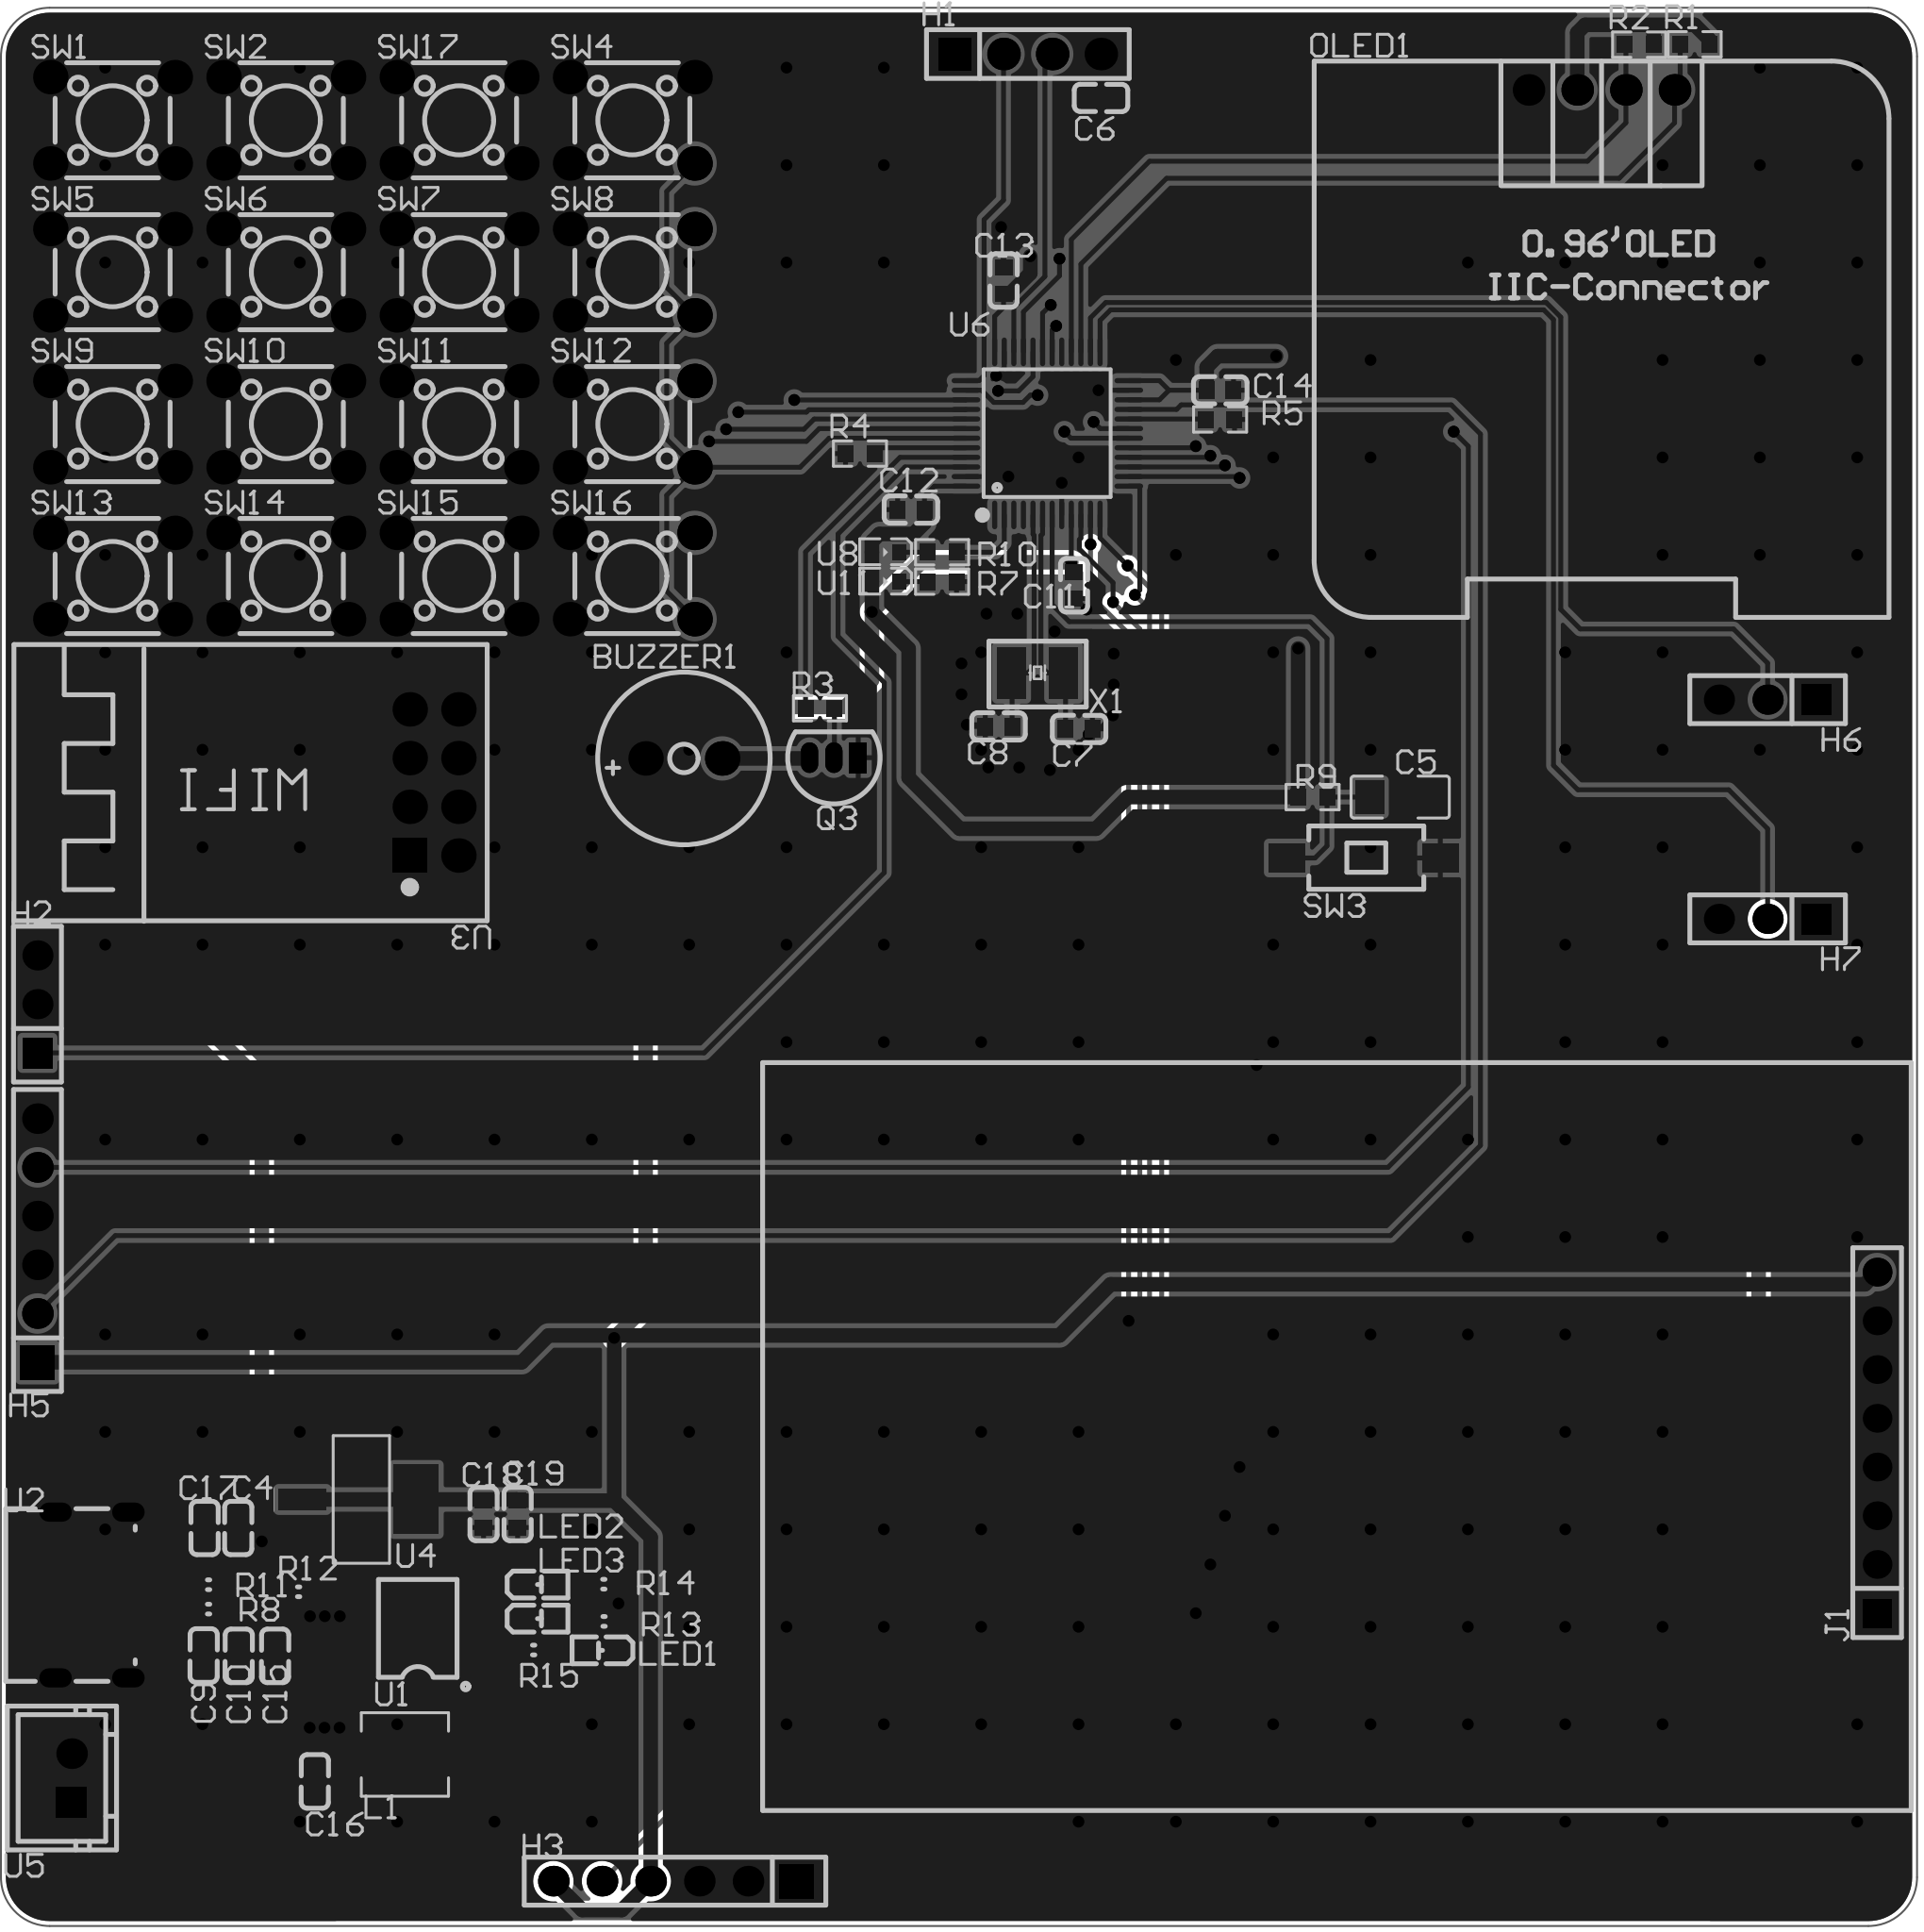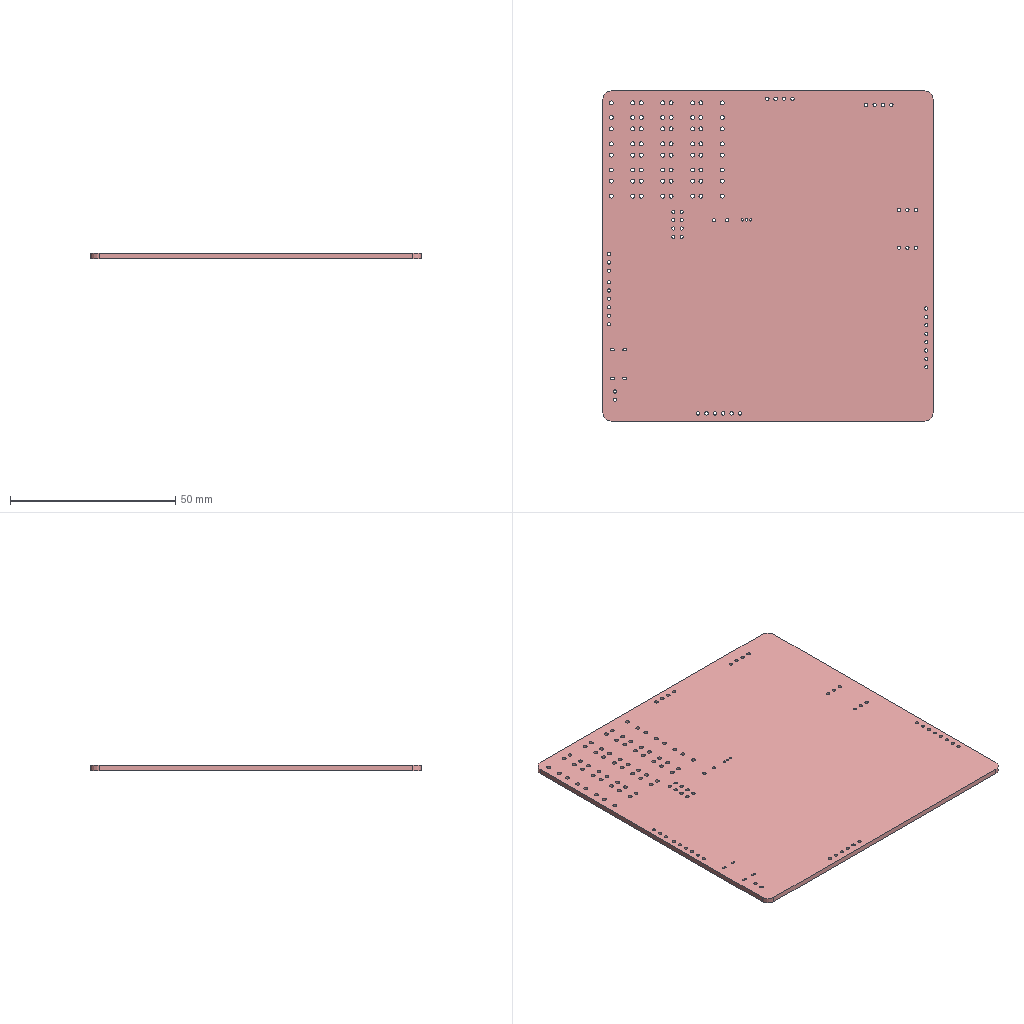Circuit board layout | Altium Designer | box 100 x 100 x 1.6 mm
Layer stack:
# Altium Designer layer stack of  (unit mm; dielectric type: 0 none, 1 core, 2 prepreg, 3 surface material)
index,name,kind,layer,copper_thickness_mm,dielectric_type,dielectric_thickness_mm,dielectric_material,dielectric_constant
0,Top Paste Mask Layer,other,,,,,,
1,Top Silkscreen Layer,other,,,,,,
2,Top Solder Mask Layer,dielectric,,,3,0.01,,3.3
3,Top Layer,copper,Top Layer,0.035,,,,
4,Dielectric1,dielectric,,,3,1.51,FR4,4.5
5,Bottom Layer,copper,Bottom Layer,0.035,,,,
6,Bottom Solder Mask Layer,dielectric,,,3,0.01,,3.3
7,Bottom Silkscreen Layer,other,,,,,,
8,Bottom Paste Mask Layer,other,,,,,,
# drill layer pairs: low layer,high layer
drill_pair,Top Layer,Bottom Layer
Part placement:
Designator,Comment,Layer,Footprint,Center-X(mm),Center-Y(mm),Rotation
BUZZER1,2.7kHz,TopLayer,BUZ-TH_BD9.0-P4.00-D0.6-FD,115.399,144.382,0
C4,10uF,TopLayer,C0603,92.139,104.263,270
C5,100uF,TopLayer,C1206,152.781,142.367,180
C6,100nF,TopLayer,C0603,137.16,178.816,180
C7,20pF,TopLayer,C0603,136.017,145.923,180
C8,20pF,TopLayer,C0603,131.826,146.05,0
C9,22uF,TopLayer,C0603,90.337,97.623,90
C10,22uF,TopLayer,C0603,92.167,97.605,90
C11,100nF,TopLayer,C0603,135.763,153.416,90
C12,100nF,TopLayer,C0603,127.254,157.353,0
C13,100nF,TopLayer,C0603,132.08,169.291,270
C14,100nF,TopLayer,C0603,143.383,163.576,180
C15,22uF,TopLayer,C0603,94.066,97.605,90
C16,22uF,TopLayer,C0603,96.139,91.059,90
C17,100nF,TopLayer,C0603,90.383,104.263,270
C18,10uF,TopLayer,C0603,104.942,104.989,90
C19,100nF,TopLayer,C0603,106.72,104.989,90
H1,,TopLayer,HDR-TH_4P-P2.54-V-F,133.35,181.102,0
H2,,TopLayer,HDR-TH_3P-P2.54-V-F,81.661,131.572,90
H3,,TopLayer,HDR-TH_6P-P2.54-V-F,114.935,85.852,180
H5,,TopLayer,HDR-TH_6P-P2.54-V-F,81.661,119.253,90
J1,,TopLayer,HDR-TH_8P-P2.54-V-M,177.673,108.712,90
L1,2.2uH,TopLayer,IND-SMD_L4.4-W4.2,100.838,92.456,180
LED1,Battery,TopLayer,LED0603_L1.6-W0.8-RD_BLUE,111.033,97.885,180
LED2,Discharge,TopLayer,LED0603_L1.6-W0.8-RD_BLUE,107.874,101.316,0
LED3,Charge,TopLayer,LED0603_L1.6-W0.8-RD_BLUE,107.874,99.538,0
OLED1,,TopLayer,0.96OLED_4P,163.291,179.234,0
Q3,,TopLayer,S8050_TO_92,123.226,144.422,180
R1,5.1K,TopLayer,R0603,168.148,181.61,0
R2,5.1K,TopLayer,R0603,165.252,181.593,0
R4,10kΩ,TopLayer,R0603,124.587,160.274,0
R5,10kΩ,TopLayer,R0603,143.383,162.052,180
R7,510Ω,TopLayer,R0603,128.875,153.599,0
R8,5.1K,TopLayer,R0603-NSK,90.591,100.036,180
R9,1kΩ,TopLayer,R0603,148.209,142.367,180
R10,510Ω,TopLayer,R0603,128.875,155.131,0
R11,5.1K,TopLayer,R0603-NSK,90.591,101.306,180
R12,56K,TopLayer,R0603-NSK,95.29,100.937,180
R13,5.1K,TopLayer,R0603-NSK,111.232,99.394,180
R14,5.1K,TopLayer,R0603-NSK,111.218,101.333,180
R15,5.1K,TopLayer,R0603-NSK,107.557,97.901,180
SW1,KH-6X6X6H-TJ,TopLayer,SW-TH_4P-L6.0-W6.0-P4.50-LS6.5,85.583,177.649,0
SW2,KH-6X6X6H-TJ,TopLayer,SW-TH_4P-L6.0-W6.0-P4.50-LS6.5,94.624,177.649,0
SW3,TS-1101-C-W,TopLayer,SW-SMD_L6.0-W3.3-LS8.0,150.876,139.192,180
SW4,KH-6X6X6H-TJ,TopLayer,SW-TH_4P-L6.0-W6.0-P4.50-LS6.5,112.707,177.649,0
SW5,KH-6X6X6H-TJ,TopLayer,SW-TH_4P-L6.0-W6.0-P4.50-LS6.5,85.583,169.73,0
SW6,KH-6X6X6H-TJ,TopLayer,SW-TH_4P-L6.0-W6.0-P4.50-LS6.5,94.624,169.73,0
SW7,KH-6X6X6H-TJ,TopLayer,SW-TH_4P-L6.0-W6.0-P4.50-LS6.5,103.666,169.73,0
SW8,KH-6X6X6H-TJ,TopLayer,SW-TH_4P-L6.0-W6.0-P4.50-LS6.5,112.707,169.73,0
SW9,KH-6X6X6H-TJ,TopLayer,SW-TH_4P-L6.0-W6.0-P4.50-LS6.5,85.583,161.81,0
SW10,KH-6X6X6H-TJ,TopLayer,SW-TH_4P-L6.0-W6.0-P4.50-LS6.5,94.624,161.81,0
SW11,KH-6X6X6H-TJ,TopLayer,SW-TH_4P-L6.0-W6.0-P4.50-LS6.5,103.666,161.81,0
SW12,KH-6X6X6H-TJ,TopLayer,SW-TH_4P-L6.0-W6.0-P4.50-LS6.5,112.707,161.81,0
SW13,KH-6X6X6H-TJ,TopLayer,SW-TH_4P-L6.0-W6.0-P4.50-LS6.5,85.583,153.892,0
SW14,KH-6X6X6H-TJ,TopLayer,SW-TH_4P-L6.0-W6.0-P4.50-LS6.5,94.624,153.892,0
SW15,KH-6X6X6H-TJ,TopLayer,SW-TH_4P-L6.0-W6.0-P4.50-LS6.5,103.666,153.892,0
SW16,KH-6X6X6H-TJ,TopLayer,SW-TH_4P-L6.0-W6.0-P4.50-LS6.5,112.707,153.892,0
SW17,KH-6X6X6H-TJ,TopLayer,SW-TH_4P-L6.0-W6.0-P4.50-LS6.5,103.666,177.649,0
U1,ETA9742,TopLayer,ESOP-8_L4.9-W3.9-P1.27-LS6.0-BL-EP,101.508,99.03,90
U2,YTC-TC6-268,TopLayer,TYPE-C-SMD_YIYUAN_YTC-TC6-268,84.731,100.77,270
U4,AMS1117-3.3,TopLayer,SOT-223-3_L6.5-W3.4-P2.30-LS7.0-BR,98.465,105.751,180
U6,STM32F103C8T6,TopLayer,LQFP-48_L7.0-W7.0-P0.50-LS9.0-BL,134.367,161.326,0
U8,42-51/GHC-YW2X2K/3T,TopLayer,LED-SMD_L1.6-W0.8-FD_GREEN-1,125.925,155.131,0
U11,42-51/GHC-YW2X2K/3T,TopLayer,LED-SMD_L1.6-W0.8-FD_GREEN-1,125.925,153.599,0
X1,8MHz,TopLayer,CRYSTAL-SMD_L3.2-W2.5_3225-8MHZ,133.858,148.844,180
R3,1K,TopLayer,R0603,122.501,146.998,180
U5,_x001F_XH2.54-2P,TopLayer,CONN-TH_2P-P2.54-V,83.445,91.23,90
H6,,TopLayer,HDR-TH_3P-P2.54-V-F,171.958,147.447,180
H7,,TopLayer,HDR-TH_3P-P2.54-V-F,171.958,136.017,180
U3,2.4GHz,TopLayer,WIFIM-TH_8P-L24.7-W14.4-P2.54,102.362,143.129,180
Pad and via stacks:
# Altium Designer via and pad stacks of  (unit mm). Each distinct definition once, with the count of objects using it.
# via: kind,start_layer,end_layer,hole_mm,diameter_mm,mode(0 simple;1 top-mid-bottom;2 full stack),diameter_per_layer,count,example_net
# pad: kind,layer,hole_mm,hole_type(0 round;1 square;2 slot),plating,top_size,top_shape(1 round;2 rect;3 octagon;9 rounded rect),mid_size,bottom_size,mode,footprint,size_per_layer,count,example
pad,Multi-Layer,1,0,plated,1.8x1.8,1,1.8x1.8,1.8x1.8,0,BUZ-TH_BD9.0-P4.00-D0.6-FD,,2,BUZZER1.1
pad,Multi-Layer,1.1,0,plated,1.7x1.7,2,1.7x1.7,1.7x1.7,0,HDR-TH_4P-P2.54-V-F,,1,H1.1
pad,Multi-Layer,1.1,0,plated,1.7x1.7,1,1.7x1.7,1.7x1.7,0,HDR-TH_4P-P2.54-V-F,,3,H1.2
pad,Multi-Layer,1.02,0,plated,1.575x1.575,1,1.575x1.575,1.575x1.575,0,HDR-TH_3P-P2.54-V-F,,6,H2.3
pad,Multi-Layer,1.02,0,plated,1.575x1.575,2,1.575x1.575,1.575x1.575,0,HDR-TH_3P-P2.54-V-F,,3,H2.1
pad,Multi-Layer,1.02,0,plated,1.6x1.6,1,1.6x1.6,1.6x1.6,0,HDR-TH_6P-P2.54-V-F,,10,H3.6
pad,Multi-Layer,1.02,0,plated,1.8x1.8,2,1.8x1.8,1.8x1.8,0,HDR-TH_6P-P2.54-V-F,,2,H3.1
pad,Multi-Layer,1,0,plated,1.5x1.5,2,1.5x1.5,1.5x1.5,0,HDR-TH_8P-P2.54-V-M,,1,J1.1
pad,Multi-Layer,1,0,plated,1.5x1.5,1,1.5x1.5,1.5x1.5,0,HDR-TH_8P-P2.54-V-M,,7,J1.2
pad,Multi-Layer,1,0,plated,1.65x1.65,1,1.65x1.65,1.65x1.65,0,0.96OLED_4P,,4,OLED1.4
pad,Multi-Layer,0.701,0,plated,0.8992x1.6,2,0.8992x1.6,0.8992x1.6,0,S8050_TO_92,,1,Q3.1
pad,Multi-Layer,0.701,0,plated,0.8992x1.6,1,0.8992x1.6,0.8992x1.6,0,S8050_TO_92,,2,Q3.2
pad,Multi-Layer,1.2,0,plated,1.8x1.8,1,1.8x1.8,1.8x1.8,0,SW-TH_4P-L6.0-W6.0-P4.50-LS6.5,,64,SW1.1
pad,Multi-Layer,0.6,2,plated,1x1.7,1,1x1.7,1x1.7,0,TYPE-C-SMD_YIYUAN_YTC-TC6-268,,4,U2.3
pad,Multi-Layer,1,0,plated,1.6x1.6,1,1.6x1.6,1.6x1.6,0,CONN-TH_2P-P2.54-V,,1,U5.2
pad,Multi-Layer,1,0,plated,1.6x1.6,2,1.6x1.6,1.6x1.6,0,CONN-TH_2P-P2.54-V,,1,U5.1
pad,Multi-Layer,1,0,plated,1.8x1.8,1,1.8x1.8,1.8x1.8,0,WIFIM-TH_8P-L24.7-W14.4-P2.54,,7,U3.8
pad,Multi-Layer,1,0,plated,1.8x1.8,2,1.8x1.8,1.8x1.8,0,WIFIM-TH_8P-L24.7-W14.4-P2.54,,1,U3.1
pad,Top Layer,0,0,plated,0.8x0.9,2,0.8x0.9,0.8x0.9,0,C0603,,30,C4.2
pad,Top Layer,0,0,plated,1.485x1.728,2,1.485x1.728,1.485x1.728,0,C1206,,2,C5.2
pad,Top Layer,0,0,plated,1.4x2.12,2,1.4x2.12,1.4x2.12,0,IND-SMD_L4.4-W4.2,,2,L1.1
pad,Top Layer,0,0,plated,0.8x0.8,2,0.8x0.8,0.8x0.8,0,LED0603_L1.6-W0.8-RD_BLUE,,6,LED1.2
pad,Top Layer,0,0,plated,0.8065x0.864,2,0.8065x0.864,0.8065x0.864,0,R0603,,16,R1.2
pad,Top Layer,0,0,plated,0.8065x0.864,2,0.8065x0.864,0.8065x0.864,0,R0603-NSK,,12,R8.2
pad,Top Layer,0,0,plated,1.9x1.5,2,1.9x1.5,1.9x1.5,0,SW-SMD_L6.0-W3.3-LS8.0,,2,SW3.1
pad,Top Layer,0,0,plated,0.6x1.2,2,0.6x1.2,0.6x1.2,0,ESOP-8_L4.9-W3.9-P1.27-LS6.0-BL-EP,,8,U1.1
pad,Top Layer,0,0,plated,3.5x2.5,2,3.5x2.5,3.5x2.5,0,ESOP-8_L4.9-W3.9-P1.27-LS6.0-BL-EP,,1,U1.9
pad,Top Layer,0,0,plated,0.8x1.6,2,0.8x1.6,0.8x1.6,0,TYPE-C-SMD_YIYUAN_YTC-TC6-268,,2,U2.A12
pad,Top Layer,0,0,plated,0.76x1.6,2,0.76x1.6,0.76x1.6,0,TYPE-C-SMD_YIYUAN_YTC-TC6-268,,2,U2.A9
pad,Top Layer,0,0,plated,0.7x1.6,2,0.7x1.6,0.7x1.6,0,TYPE-C-SMD_YIYUAN_YTC-TC6-268,,2,U2.B5
pad,Top Layer,0,0,plated,2.5x1.1,2,2.5x1.1,2.5x1.1,0,SOT-223-3_L6.5-W3.4-P2.30-LS7.0-BR,,3,U4.1
pad,Top Layer,0,0,plated,2.34x3.6,2,2.34x3.6,2.34x3.6,0,SOT-223-3_L6.5-W3.4-P2.30-LS7.0-BR,,1,U4.4
pad,Top Layer,0,0,plated,0.27x1.5,1,0.27x1.5,0.27x1.5,0,LQFP-48_L7.0-W7.0-P0.50-LS9.0-BL,,24,U6.1
pad,Top Layer,0,0,plated,1.5x0.27,1,1.5x0.27,1.5x0.27,0,LQFP-48_L7.0-W7.0-P0.50-LS9.0-BL,,24,U6.13
pad,Top Layer,0,0,plated,0.8x0.7,2,0.8x0.7,0.8x0.7,0,LED-SMD_L1.6-W0.8-FD_GREEN-1,,4,U8.1
pad,Top Layer,0,0,plated,1.524x2.7,2,1.524x2.7,1.524x2.7,0,CRYSTAL-SMD_L3.2-W2.5_3225-8MHZ,,2,X1.1
via,Top Layer,Bottom Layer,0.3048,0.61,0,,270,MFR_RST
Copper pours:
name,layer,net,type(0 solid;1 hatched;2 none)
Top Layer-GND,Top Layer,GND,0
Bottom Layer-GND,Bottom Layer,GND,0